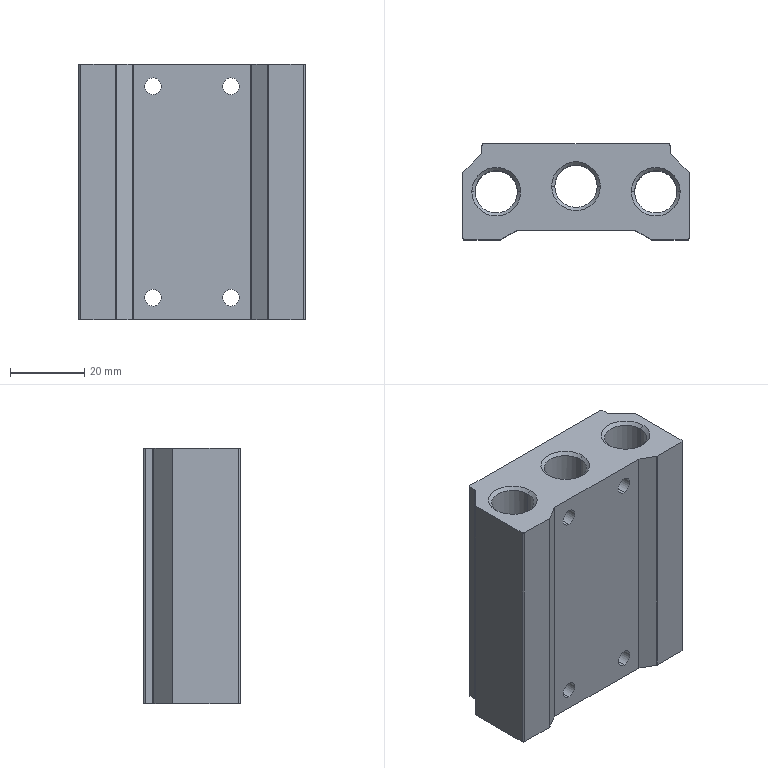Part | STEP file | 200M-2F | 1 solid | 90 faces | box 61 x 26 x 69 mm | volume 73969 mm3 | cylinder 44 | cone 28 | plane 18 | commonest cylinder face diameters 1 x10 2.459 x8 4.5 x8 6.5 x8 11.445 x6 10.2 x4